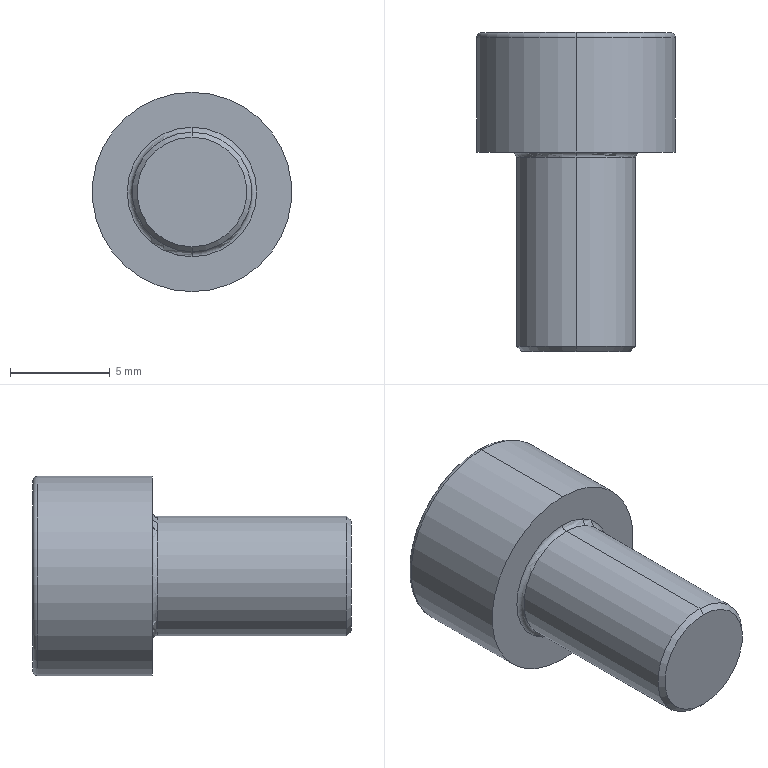Part | STEP file | 1 solid | 20 faces | box 10 x 16 x 10 mm | volume 688.299 mm3 | plane 10 | torus 4 | cylinder 4 | cone 2 | commonest cylinder face diameters 6 x2 10 x2
STEP:
#1=CARTESIAN_POINT('',(0.,-10.,-2.75));
#2=VERTEX_POINT('',#1);
#3=CARTESIAN_POINT('',(0.,-10.,2.75));
#4=VERTEX_POINT('',#3);
#5=CARTESIAN_POINT('',(0.,-10.,0.));
#6=DIRECTION('',(0.,-1.,0.));
#7=DIRECTION('',(0.,0.,-1.));
#8=AXIS2_PLACEMENT_3D('',#5,#6,#7);
#9=CIRCLE('',#8,2.75);
#10=EDGE_CURVE('',#2,#4,#9,.T.);
#11=ORIENTED_EDGE('',*,*,#10,.F.);
#12=CARTESIAN_POINT('',(0.,-9.75,-3.));
#13=VERTEX_POINT('',#12);
#14=CARTESIAN_POINT('',(0.,-10.,-2.75));
#15=DIRECTION('',(0.,0.7071,-0.7071));
#16=VECTOR('',#15,1000.);
#17=LINE('',#14,#16);
#18=EDGE_CURVE('',#2,#13,#17,.T.);
#19=ORIENTED_EDGE('',*,*,#18,.T.);
#20=CARTESIAN_POINT('',(0.,-9.75,3.));
#21=VERTEX_POINT('',#20);
#22=CARTESIAN_POINT('',(0.,-9.75,0.));
#23=DIRECTION('',(0.,1.,0.));
#24=DIRECTION('',(0.,0.,-1.));
#25=AXIS2_PLACEMENT_3D('',#22,#23,#24);
#26=CIRCLE('',#25,3.);
#27=EDGE_CURVE('',#21,#13,#26,.T.);
#28=ORIENTED_EDGE('',*,*,#27,.F.);
#29=CARTESIAN_POINT('',(0.,-10.,2.75));
#30=DIRECTION('',(0.,0.7071,0.7071));
#31=VECTOR('',#30,1000.);
#32=LINE('',#29,#31);
#33=EDGE_CURVE('',#4,#21,#32,.T.);
#34=ORIENTED_EDGE('',*,*,#33,.F.);
#35=EDGE_LOOP('',(#11,#19,#28,#34));
#36=FACE_OUTER_BOUND('',#35,.T.);
#37=CARTESIAN_POINT('',(0.,-10.,0.));
#38=DIRECTION('',(0.,1.,0.));
#39=DIRECTION('',(0.,0.,1.));
#40=AXIS2_PLACEMENT_3D('',#37,#38,#39);
#41=CONICAL_SURFACE('',#40,2.75,0.7854);
#42=ADVANCED_FACE('',(#36),#41,.T.);
#43=CARTESIAN_POINT('',(0.,5.75,-5.));
#44=VERTEX_POINT('',#43);
#45=CARTESIAN_POINT('',(0.,5.75,5.));
#46=VERTEX_POINT('',#45);
#47=CARTESIAN_POINT('',(0.,5.75,0.));
#48=DIRECTION('',(0.,-1.,0.));
#49=DIRECTION('',(0.,0.,1.));
#50=AXIS2_PLACEMENT_3D('',#47,#48,#49);
#51=CIRCLE('',#50,5.);
#52=EDGE_CURVE('',#44,#46,#51,.T.);
#53=ORIENTED_EDGE('',*,*,#52,.F.);
#54=CARTESIAN_POINT('',(0.,6.,-4.75));
#55=VERTEX_POINT('',#54);
#56=CARTESIAN_POINT('',(0.,5.75,-4.75));
#57=DIRECTION('',(1.,0.,0.));
#58=DIRECTION('',(0.,0.,-1.));
#59=AXIS2_PLACEMENT_3D('',#56,#57,#58);
#60=CIRCLE('',#59,0.25);
#61=EDGE_CURVE('',#44,#55,#60,.T.);
#62=ORIENTED_EDGE('',*,*,#61,.T.);
#63=CARTESIAN_POINT('',(0.,6.,4.75));
#64=VERTEX_POINT('',#63);
#65=CARTESIAN_POINT('',(0.,6.,0.));
#66=DIRECTION('',(0.,1.,0.));
#67=DIRECTION('',(0.,0.,1.));
#68=AXIS2_PLACEMENT_3D('',#65,#66,#67);
#69=CIRCLE('',#68,4.75);
#70=EDGE_CURVE('',#64,#55,#69,.T.);
#71=ORIENTED_EDGE('',*,*,#70,.F.);
#72=CARTESIAN_POINT('',(0.,5.75,4.75));
#73=DIRECTION('',(-1.,0.,0.));
#74=DIRECTION('',(0.,0.,1.));
#75=AXIS2_PLACEMENT_3D('',#72,#73,#74);
#76=CIRCLE('',#75,0.25);
#77=EDGE_CURVE('',#46,#64,#76,.T.);
#78=ORIENTED_EDGE('',*,*,#77,.F.);
#79=EDGE_LOOP('',(#53,#62,#71,#78));
#80=FACE_OUTER_BOUND('',#79,.T.);
#81=CARTESIAN_POINT('',(0.,5.75,0.));
#82=DIRECTION('',(0.,1.,0.));
#83=DIRECTION('',(0.,0.,1.));
#84=AXIS2_PLACEMENT_3D('',#81,#82,#83);
#85=TOROIDAL_SURFACE('',#84,4.75,0.25);
#86=ADVANCED_FACE('',(#80),#85,.T.);
#87=CARTESIAN_POINT('',(0.,-0.25,3.));
#88=VERTEX_POINT('',#87);
#89=CARTESIAN_POINT('',(0.,-0.25,-3.));
#90=VERTEX_POINT('',#89);
#91=CARTESIAN_POINT('',(0.,-0.25,0.));
#92=DIRECTION('',(0.,-1.,0.));
#93=DIRECTION('',(0.,0.,-1.));
#94=AXIS2_PLACEMENT_3D('',#91,#92,#93);
#95=CIRCLE('',#94,3.);
#96=EDGE_CURVE('',#88,#90,#95,.T.);
#97=ORIENTED_EDGE('',*,*,#96,.F.);
#98=CARTESIAN_POINT('',(0.,0.,3.25));
#99=VERTEX_POINT('',#98);
#100=CARTESIAN_POINT('',(0.,-0.25,3.25));
#101=DIRECTION('',(1.,0.,0.));
#102=DIRECTION('',(0.,0.,-1.));
#103=AXIS2_PLACEMENT_3D('',#100,#101,#102);
#104=CIRCLE('',#103,0.25);
#105=EDGE_CURVE('',#88,#99,#104,.T.);
#106=ORIENTED_EDGE('',*,*,#105,.T.);
#107=CARTESIAN_POINT('',(0.,0.,-3.25));
#108=VERTEX_POINT('',#107);
#109=CARTESIAN_POINT('',(0.,0.,0.));
#110=DIRECTION('',(0.,1.,0.));
#111=DIRECTION('',(0.,0.,-1.));
#112=AXIS2_PLACEMENT_3D('',#109,#110,#111);
#113=CIRCLE('',#112,3.25);
#114=EDGE_CURVE('',#108,#99,#113,.T.);
#115=ORIENTED_EDGE('',*,*,#114,.F.);
#116=CARTESIAN_POINT('',(0.,-0.25,-3.25));
#117=DIRECTION('',(-1.,0.,0.));
#118=DIRECTION('',(0.,0.,1.));
#119=AXIS2_PLACEMENT_3D('',#116,#117,#118);
#120=CIRCLE('',#119,0.25);
#121=EDGE_CURVE('',#90,#108,#120,.T.);
#122=ORIENTED_EDGE('',*,*,#121,.F.);
#123=EDGE_LOOP('',(#97,#106,#115,#122));
#124=FACE_OUTER_BOUND('',#123,.T.);
#125=CARTESIAN_POINT('',(0.,-0.25,0.));
#126=DIRECTION('',(0.,-1.,0.));
#127=DIRECTION('',(0.,0.,-1.));
#128=AXIS2_PLACEMENT_3D('',#125,#126,#127);
#129=TOROIDAL_SURFACE('',#128,3.25,0.25);
#130=ADVANCED_FACE('',(#124),#129,.F.);
#131=CARTESIAN_POINT('',(0.,-0.25,0.));
#132=DIRECTION('',(0.,-1.,0.));
#133=DIRECTION('',(0.,0.,-1.));
#134=AXIS2_PLACEMENT_3D('',#131,#132,#133);
#135=CIRCLE('',#134,3.);
#136=EDGE_CURVE('',#90,#88,#135,.T.);
#137=ORIENTED_EDGE('',*,*,#136,.T.);
#138=CARTESIAN_POINT('',(0.,0.,3.));
#139=DIRECTION('',(0.,-1.,0.));
#140=VECTOR('',#139,1000.);
#141=LINE('',#138,#140);
#142=EDGE_CURVE('',#88,#21,#141,.T.);
#143=ORIENTED_EDGE('',*,*,#142,.T.);
#144=ORIENTED_EDGE('',*,*,#27,.T.);
#145=CARTESIAN_POINT('',(0.,0.,-3.));
#146=DIRECTION('',(0.,-1.,0.));
#147=VECTOR('',#146,1000.);
#148=LINE('',#145,#147);
#149=EDGE_CURVE('',#90,#13,#148,.T.);
#150=ORIENTED_EDGE('',*,*,#149,.F.);
#151=EDGE_LOOP('',(#137,#143,#144,#150));
#152=FACE_OUTER_BOUND('',#151,.T.);
#153=CARTESIAN_POINT('',(0.,0.,0.));
#154=DIRECTION('',(0.,-1.,0.));
#155=DIRECTION('',(0.,0.,-1.));
#156=AXIS2_PLACEMENT_3D('',#153,#154,#155);
#157=CYLINDRICAL_SURFACE('',#156,3.);
#158=ADVANCED_FACE('',(#152),#157,.T.);
#159=ORIENTED_EDGE('',*,*,#52,.T.);
#160=CARTESIAN_POINT('',(0.,0.,5.));
#161=VERTEX_POINT('',#160);
#162=CARTESIAN_POINT('',(0.,0.,5.));
#163=DIRECTION('',(0.,-1.,0.));
#164=VECTOR('',#163,1000.);
#165=LINE('',#162,#164);
#166=EDGE_CURVE('',#46,#161,#165,.T.);
#167=ORIENTED_EDGE('',*,*,#166,.T.);
#168=CARTESIAN_POINT('',(0.,0.,-5.));
#169=VERTEX_POINT('',#168);
#170=CARTESIAN_POINT('',(0.,0.,0.));
#171=DIRECTION('',(0.,-1.,0.));
#172=DIRECTION('',(0.,0.,-1.));
#173=AXIS2_PLACEMENT_3D('',#170,#171,#172);
#174=CIRCLE('',#173,5.);
#175=EDGE_CURVE('',#169,#161,#174,.T.);
#176=ORIENTED_EDGE('',*,*,#175,.F.);
#177=CARTESIAN_POINT('',(0.,0.,-5.));
#178=DIRECTION('',(0.,-1.,0.));
#179=VECTOR('',#178,1000.);
#180=LINE('',#177,#179);
#181=EDGE_CURVE('',#44,#169,#180,.T.);
#182=ORIENTED_EDGE('',*,*,#181,.F.);
#183=EDGE_LOOP('',(#159,#167,#176,#182));
#184=FACE_OUTER_BOUND('',#183,.T.);
#185=CARTESIAN_POINT('',(0.,0.,0.));
#186=DIRECTION('',(0.,-1.,0.));
#187=DIRECTION('',(0.,0.,-1.));
#188=AXIS2_PLACEMENT_3D('',#185,#186,#187);
#189=CYLINDRICAL_SURFACE('',#188,5.);
#190=ADVANCED_FACE('',(#184),#189,.T.);
#191=ORIENTED_EDGE('',*,*,#70,.T.);
#192=CARTESIAN_POINT('',(0.,6.,0.));
#193=DIRECTION('',(0.,1.,0.));
#194=DIRECTION('',(0.,0.,1.));
#195=AXIS2_PLACEMENT_3D('',#192,#193,#194);
#196=CIRCLE('',#195,4.75);
#197=EDGE_CURVE('',#55,#64,#196,.T.);
#198=ORIENTED_EDGE('',*,*,#197,.T.);
#199=EDGE_LOOP('',(#191,#198));
#200=FACE_OUTER_BOUND('',#199,.T.);
#201=CARTESIAN_POINT('',(0.,6.,-2.887));
#202=VERTEX_POINT('',#201);
#203=CARTESIAN_POINT('',(-2.5,6.,-1.443));
#204=VERTEX_POINT('',#203);
#205=CARTESIAN_POINT('',(0.,6.,-2.887));
#206=DIRECTION('',(-0.866,0.,0.5));
#207=VECTOR('',#206,1000.);
#208=LINE('',#205,#207);
#209=EDGE_CURVE('',#202,#204,#208,.T.);
#210=ORIENTED_EDGE('',*,*,#209,.F.);
#211=CARTESIAN_POINT('',(2.5,6.,-1.443));
#212=VERTEX_POINT('',#211);
#213=CARTESIAN_POINT('',(2.5,6.,-1.443));
#214=DIRECTION('',(-0.866,0.,-0.5));
#215=VECTOR('',#214,1000.);
#216=LINE('',#213,#215);
#217=EDGE_CURVE('',#212,#202,#216,.T.);
#218=ORIENTED_EDGE('',*,*,#217,.F.);
#219=CARTESIAN_POINT('',(2.5,6.,1.443));
#220=VERTEX_POINT('',#219);
#221=CARTESIAN_POINT('',(2.5,6.,1.443));
#222=DIRECTION('',(0.,0.,-1.));
#223=VECTOR('',#222,1000.);
#224=LINE('',#221,#223);
#225=EDGE_CURVE('',#220,#212,#224,.T.);
#226=ORIENTED_EDGE('',*,*,#225,.F.);
#227=CARTESIAN_POINT('',(0.,6.,2.887));
#228=VERTEX_POINT('',#227);
#229=CARTESIAN_POINT('',(0.,6.,2.887));
#230=DIRECTION('',(0.866,0.,-0.5));
#231=VECTOR('',#230,1000.);
#232=LINE('',#229,#231);
#233=EDGE_CURVE('',#228,#220,#232,.T.);
#234=ORIENTED_EDGE('',*,*,#233,.F.);
#235=CARTESIAN_POINT('',(-2.5,6.,1.443));
#236=VERTEX_POINT('',#235);
#237=CARTESIAN_POINT('',(-2.5,6.,1.443));
#238=DIRECTION('',(0.866,0.,0.5));
#239=VECTOR('',#238,1000.);
#240=LINE('',#237,#239);
#241=EDGE_CURVE('',#236,#228,#240,.T.);
#242=ORIENTED_EDGE('',*,*,#241,.F.);
#243=CARTESIAN_POINT('',(-2.5,6.,-1.443));
#244=DIRECTION('',(0.,0.,1.));
#245=VECTOR('',#244,1000.);
#246=LINE('',#243,#245);
#247=EDGE_CURVE('',#204,#236,#246,.T.);
#248=ORIENTED_EDGE('',*,*,#247,.F.);
#249=EDGE_LOOP('',(#210,#218,#226,#234,#242,#248));
#250=FACE_BOUND('',#249,.T.);
#251=CARTESIAN_POINT('',(0.,6.,0.));
#252=DIRECTION('',(0.,1.,0.));
#253=DIRECTION('',(0.,0.,1.));
#254=AXIS2_PLACEMENT_3D('',#251,#252,#253);
#255=PLANE('',#254);
#256=ADVANCED_FACE('',(#200,#250),#255,.T.);
#257=ORIENTED_EDGE('',*,*,#166,.F.);
#258=CARTESIAN_POINT('',(0.,5.75,0.));
#259=DIRECTION('',(0.,-1.,0.));
#260=DIRECTION('',(0.,0.,1.));
#261=AXIS2_PLACEMENT_3D('',#258,#259,#260);
#262=CIRCLE('',#261,5.);
#263=EDGE_CURVE('',#46,#44,#262,.T.);
#264=ORIENTED_EDGE('',*,*,#263,.T.);
#265=ORIENTED_EDGE('',*,*,#181,.T.);
#266=CARTESIAN_POINT('',(0.,0.,0.));
#267=DIRECTION('',(0.,-1.,0.));
#268=DIRECTION('',(0.,0.,-1.));
#269=AXIS2_PLACEMENT_3D('',#266,#267,#268);
#270=CIRCLE('',#269,5.);
#271=EDGE_CURVE('',#161,#169,#270,.T.);
#272=ORIENTED_EDGE('',*,*,#271,.F.);
#273=EDGE_LOOP('',(#257,#264,#265,#272));
#274=FACE_OUTER_BOUND('',#273,.T.);
#275=CARTESIAN_POINT('',(0.,0.,0.));
#276=DIRECTION('',(0.,-1.,0.));
#277=DIRECTION('',(0.,0.,-1.));
#278=AXIS2_PLACEMENT_3D('',#275,#276,#277);
#279=CYLINDRICAL_SURFACE('',#278,5.);
#280=ADVANCED_FACE('',(#274),#279,.T.);
#281=ORIENTED_EDGE('',*,*,#114,.T.);
#282=CARTESIAN_POINT('',(0.,0.,0.));
#283=DIRECTION('',(0.,1.,0.));
#284=DIRECTION('',(0.,0.,-1.));
#285=AXIS2_PLACEMENT_3D('',#282,#283,#284);
#286=CIRCLE('',#285,3.25);
#287=EDGE_CURVE('',#99,#108,#286,.T.);
#288=ORIENTED_EDGE('',*,*,#287,.T.);
#289=EDGE_LOOP('',(#281,#288));
#290=FACE_BOUND('',#289,.T.);
#291=ORIENTED_EDGE('',*,*,#175,.T.);
#292=ORIENTED_EDGE('',*,*,#271,.T.);
#293=EDGE_LOOP('',(#291,#292));
#294=FACE_OUTER_BOUND('',#293,.T.);
#295=CARTESIAN_POINT('',(5.,0.,0.));
#296=DIRECTION('',(0.,-1.,0.));
#297=DIRECTION('',(0.,0.,-1.));
#298=AXIS2_PLACEMENT_3D('',#295,#296,#297);
#299=PLANE('',#298);
#300=ADVANCED_FACE('',(#290,#294),#299,.T.);
#301=ORIENTED_EDGE('',*,*,#142,.F.);
#302=ORIENTED_EDGE('',*,*,#96,.T.);
#303=ORIENTED_EDGE('',*,*,#149,.T.);
#304=CARTESIAN_POINT('',(0.,-9.75,0.));
#305=DIRECTION('',(0.,1.,0.));
#306=DIRECTION('',(0.,0.,-1.));
#307=AXIS2_PLACEMENT_3D('',#304,#305,#306);
#308=CIRCLE('',#307,3.);
#309=EDGE_CURVE('',#13,#21,#308,.T.);
#310=ORIENTED_EDGE('',*,*,#309,.T.);
#311=EDGE_LOOP('',(#301,#302,#303,#310));
#312=FACE_OUTER_BOUND('',#311,.T.);
#313=CARTESIAN_POINT('',(0.,0.,0.));
#314=DIRECTION('',(0.,-1.,0.));
#315=DIRECTION('',(0.,0.,-1.));
#316=AXIS2_PLACEMENT_3D('',#313,#314,#315);
#317=CYLINDRICAL_SURFACE('',#316,3.);
#318=ADVANCED_FACE('',(#312),#317,.T.);
#319=CARTESIAN_POINT('',(0.,-10.,0.));
#320=DIRECTION('',(0.,-1.,0.));
#321=DIRECTION('',(0.,0.,-1.));
#322=AXIS2_PLACEMENT_3D('',#319,#320,#321);
#323=CIRCLE('',#322,2.75);
#324=EDGE_CURVE('',#4,#2,#323,.T.);
#325=ORIENTED_EDGE('',*,*,#324,.T.);
#326=ORIENTED_EDGE('',*,*,#10,.T.);
#327=EDGE_LOOP('',(#325,#326));
#328=FACE_OUTER_BOUND('',#327,.T.);
#329=CARTESIAN_POINT('',(3.,-10.,0.));
#330=DIRECTION('',(0.,-1.,0.));
#331=DIRECTION('',(0.,0.,-1.));
#332=AXIS2_PLACEMENT_3D('',#329,#330,#331);
#333=PLANE('',#332);
#334=ADVANCED_FACE('',(#328),#333,.T.);
#335=ORIENTED_EDGE('',*,*,#209,.T.);
#336=CARTESIAN_POINT('',(-2.5,3.,-1.443));
#337=VERTEX_POINT('',#336);
#338=CARTESIAN_POINT('',(-2.5,3.,-1.443));
#339=DIRECTION('',(0.,1.,0.));
#340=VECTOR('',#339,1000.);
#341=LINE('',#338,#340);
#342=EDGE_CURVE('',#337,#204,#341,.T.);
#343=ORIENTED_EDGE('',*,*,#342,.F.);
#344=CARTESIAN_POINT('',(0.,3.,-2.887));
#345=VERTEX_POINT('',#344);
#346=CARTESIAN_POINT('',(0.,3.,-2.887));
#347=DIRECTION('',(-0.866,0.,0.5));
#348=VECTOR('',#347,1000.);
#349=LINE('',#346,#348);
#350=EDGE_CURVE('',#345,#337,#349,.T.);
#351=ORIENTED_EDGE('',*,*,#350,.F.);
#352=CARTESIAN_POINT('',(0.,3.,-2.887));
#353=DIRECTION('',(0.,1.,0.));
#354=VECTOR('',#353,1000.);
#355=LINE('',#352,#354);
#356=EDGE_CURVE('',#345,#202,#355,.T.);
#357=ORIENTED_EDGE('',*,*,#356,.T.);
#358=EDGE_LOOP('',(#335,#343,#351,#357));
#359=FACE_OUTER_BOUND('',#358,.T.);
#360=CARTESIAN_POINT('',(0.,3.,-2.887));
#361=DIRECTION('',(-0.5,0.,-0.866));
#362=DIRECTION('',(-0.866,0.,0.5));
#363=AXIS2_PLACEMENT_3D('',#360,#361,#362);
#364=PLANE('',#363);
#365=ADVANCED_FACE('',(#359),#364,.F.);
#366=ORIENTED_EDGE('',*,*,#217,.T.);
#367=ORIENTED_EDGE('',*,*,#356,.F.);
#368=CARTESIAN_POINT('',(2.5,3.,-1.443));
#369=VERTEX_POINT('',#368);
#370=CARTESIAN_POINT('',(2.5,3.,-1.443));
#371=DIRECTION('',(-0.866,0.,-0.5));
#372=VECTOR('',#371,1000.);
#373=LINE('',#370,#372);
#374=EDGE_CURVE('',#369,#345,#373,.T.);
#375=ORIENTED_EDGE('',*,*,#374,.F.);
#376=CARTESIAN_POINT('',(2.5,3.,-1.443));
#377=DIRECTION('',(0.,1.,0.));
#378=VECTOR('',#377,1000.);
#379=LINE('',#376,#378);
#380=EDGE_CURVE('',#369,#212,#379,.T.);
#381=ORIENTED_EDGE('',*,*,#380,.T.);
#382=EDGE_LOOP('',(#366,#367,#375,#381));
#383=FACE_OUTER_BOUND('',#382,.T.);
#384=CARTESIAN_POINT('',(2.5,3.,-1.443));
#385=DIRECTION('',(0.5,0.,-0.866));
#386=DIRECTION('',(-0.866,0.,-0.5));
#387=AXIS2_PLACEMENT_3D('',#384,#385,#386);
#388=PLANE('',#387);
#389=ADVANCED_FACE('',(#383),#388,.F.);
#390=ORIENTED_EDGE('',*,*,#225,.T.);
#391=ORIENTED_EDGE('',*,*,#380,.F.);
#392=CARTESIAN_POINT('',(2.5,3.,1.443));
#393=VERTEX_POINT('',#392);
#394=CARTESIAN_POINT('',(2.5,3.,1.443));
#395=DIRECTION('',(0.,0.,-1.));
#396=VECTOR('',#395,1000.);
#397=LINE('',#394,#396);
#398=EDGE_CURVE('',#393,#369,#397,.T.);
#399=ORIENTED_EDGE('',*,*,#398,.F.);
#400=CARTESIAN_POINT('',(2.5,3.,1.443));
#401=DIRECTION('',(0.,1.,0.));
#402=VECTOR('',#401,1000.);
#403=LINE('',#400,#402);
#404=EDGE_CURVE('',#393,#220,#403,.T.);
#405=ORIENTED_EDGE('',*,*,#404,.T.);
#406=EDGE_LOOP('',(#390,#391,#399,#405));
#407=FACE_OUTER_BOUND('',#406,.T.);
#408=CARTESIAN_POINT('',(2.5,3.,1.443));
#409=DIRECTION('',(1.,0.,0.));
#410=DIRECTION('',(0.,0.,-1.));
#411=AXIS2_PLACEMENT_3D('',#408,#409,#410);
#412=PLANE('',#411);
#413=ADVANCED_FACE('',(#407),#412,.F.);
#414=ORIENTED_EDGE('',*,*,#233,.T.);
#415=ORIENTED_EDGE('',*,*,#404,.F.);
#416=CARTESIAN_POINT('',(0.,3.,2.887));
#417=VERTEX_POINT('',#416);
#418=CARTESIAN_POINT('',(0.,3.,2.887));
#419=DIRECTION('',(0.866,0.,-0.5));
#420=VECTOR('',#419,1000.);
#421=LINE('',#418,#420);
#422=EDGE_CURVE('',#417,#393,#421,.T.);
#423=ORIENTED_EDGE('',*,*,#422,.F.);
#424=CARTESIAN_POINT('',(0.,3.,2.887));
#425=DIRECTION('',(0.,1.,0.));
#426=VECTOR('',#425,1000.);
#427=LINE('',#424,#426);
#428=EDGE_CURVE('',#417,#228,#427,.T.);
#429=ORIENTED_EDGE('',*,*,#428,.T.);
#430=EDGE_LOOP('',(#414,#415,#423,#429));
#431=FACE_OUTER_BOUND('',#430,.T.);
#432=CARTESIAN_POINT('',(0.,3.,2.887));
#433=DIRECTION('',(0.5,0.,0.866));
#434=DIRECTION('',(0.866,0.,-0.5));
#435=AXIS2_PLACEMENT_3D('',#432,#433,#434);
#436=PLANE('',#435);
#437=ADVANCED_FACE('',(#431),#436,.F.);
#438=ORIENTED_EDGE('',*,*,#241,.T.);
#439=ORIENTED_EDGE('',*,*,#428,.F.);
#440=CARTESIAN_POINT('',(-2.5,3.,1.443));
#441=VERTEX_POINT('',#440);
#442=CARTESIAN_POINT('',(-2.5,3.,1.443));
#443=DIRECTION('',(0.866,0.,0.5));
#444=VECTOR('',#443,1000.);
#445=LINE('',#442,#444);
#446=EDGE_CURVE('',#441,#417,#445,.T.);
#447=ORIENTED_EDGE('',*,*,#446,.F.);
#448=CARTESIAN_POINT('',(-2.5,3.,1.443));
#449=DIRECTION('',(0.,1.,0.));
#450=VECTOR('',#449,1000.);
#451=LINE('',#448,#450);
#452=EDGE_CURVE('',#441,#236,#451,.T.);
#453=ORIENTED_EDGE('',*,*,#452,.T.);
#454=EDGE_LOOP('',(#438,#439,#447,#453));
#455=FACE_OUTER_BOUND('',#454,.T.);
#456=CARTESIAN_POINT('',(-2.5,3.,1.443));
#457=DIRECTION('',(-0.5,0.,0.866));
#458=DIRECTION('',(0.866,0.,0.5));
#459=AXIS2_PLACEMENT_3D('',#456,#457,#458);
#460=PLANE('',#459);
#461=ADVANCED_FACE('',(#455),#460,.F.);
#462=ORIENTED_EDGE('',*,*,#247,.T.);
#463=ORIENTED_EDGE('',*,*,#452,.F.);
#464=CARTESIAN_POINT('',(-2.5,3.,-1.443));
#465=DIRECTION('',(0.,0.,1.));
#466=VECTOR('',#465,1000.);
#467=LINE('',#464,#466);
#468=EDGE_CURVE('',#337,#441,#467,.T.);
#469=ORIENTED_EDGE('',*,*,#468,.F.);
#470=ORIENTED_EDGE('',*,*,#342,.T.);
#471=EDGE_LOOP('',(#462,#463,#469,#470));
#472=FACE_OUTER_BOUND('',#471,.T.);
#473=CARTESIAN_POINT('',(-2.5,3.,-1.443));
#474=DIRECTION('',(-1.,0.,0.));
#475=DIRECTION('',(0.,0.,1.));
#476=AXIS2_PLACEMENT_3D('',#473,#474,#475);
#477=PLANE('',#476);
#478=ADVANCED_FACE('',(#472),#477,.F.);
#479=ORIENTED_EDGE('',*,*,#350,.T.);
#480=ORIENTED_EDGE('',*,*,#468,.T.);
#481=ORIENTED_EDGE('',*,*,#446,.T.);
#482=ORIENTED_EDGE('',*,*,#422,.T.);
#483=ORIENTED_EDGE('',*,*,#398,.T.);
#484=ORIENTED_EDGE('',*,*,#374,.T.);
#485=EDGE_LOOP('',(#479,#480,#481,#482,#483,#484));
#486=FACE_OUTER_BOUND('',#485,.T.);
#487=CARTESIAN_POINT('',(0.,3.,0.));
#488=DIRECTION('',(0.,1.,0.));
#489=DIRECTION('',(0.,0.,1.));
#490=AXIS2_PLACEMENT_3D('',#487,#488,#489);
#491=PLANE('',#490);
#492=ADVANCED_FACE('',(#486),#491,.T.);
#493=ORIENTED_EDGE('',*,*,#105,.F.);
#494=ORIENTED_EDGE('',*,*,#136,.F.);
#495=ORIENTED_EDGE('',*,*,#121,.T.);
#496=ORIENTED_EDGE('',*,*,#287,.F.);
#497=EDGE_LOOP('',(#493,#494,#495,#496));
#498=FACE_OUTER_BOUND('',#497,.T.);
#499=CARTESIAN_POINT('',(0.,-0.25,0.));
#500=DIRECTION('',(0.,-1.,0.));
#501=DIRECTION('',(0.,0.,-1.));
#502=AXIS2_PLACEMENT_3D('',#499,#500,#501);
#503=TOROIDAL_SURFACE('',#502,3.25,0.25);
#504=ADVANCED_FACE('',(#498),#503,.F.);
#505=ORIENTED_EDGE('',*,*,#61,.F.);
#506=ORIENTED_EDGE('',*,*,#263,.F.);
#507=ORIENTED_EDGE('',*,*,#77,.T.);
#508=ORIENTED_EDGE('',*,*,#197,.F.);
#509=EDGE_LOOP('',(#505,#506,#507,#508));
#510=FACE_OUTER_BOUND('',#509,.T.);
#511=CARTESIAN_POINT('',(0.,5.75,0.));
#512=DIRECTION('',(0.,1.,0.));
#513=DIRECTION('',(0.,0.,1.));
#514=AXIS2_PLACEMENT_3D('',#511,#512,#513);
#515=TOROIDAL_SURFACE('',#514,4.75,0.25);
#516=ADVANCED_FACE('',(#510),#515,.T.);
#517=ORIENTED_EDGE('',*,*,#18,.F.);
#518=ORIENTED_EDGE('',*,*,#324,.F.);
#519=ORIENTED_EDGE('',*,*,#33,.T.);
#520=ORIENTED_EDGE('',*,*,#309,.F.);
#521=EDGE_LOOP('',(#517,#518,#519,#520));
#522=FACE_OUTER_BOUND('',#521,.T.);
#523=CARTESIAN_POINT('',(0.,-10.,0.));
#524=DIRECTION('',(0.,1.,0.));
#525=DIRECTION('',(0.,0.,1.));
#526=AXIS2_PLACEMENT_3D('',#523,#524,#525);
#527=CONICAL_SURFACE('',#526,2.75,0.7854);
#528=ADVANCED_FACE('',(#522),#527,.T.);
#529=CLOSED_SHELL('',(#42,#86,#130,#158,#190,#256,#280,#300,#318,#334,#365,#389,#413,#437,#461,#478,#492,#504,#516,#528));
#530=MANIFOLD_SOLID_BREP('',#529);
#531=CARTESIAN_POINT('',(0.,0.,0.));
#532=DIRECTION('',(0.,0.,1.));
#533=DIRECTION('',(1.,0.,0.));
#534=AXIS2_PLACEMENT_3D('',#531,#532,#533);
#535=(LENGTH_UNIT()NAMED_UNIT(*)SI_UNIT(.MILLI.,.METRE.));
#536=UNCERTAINTY_MEASURE_WITH_UNIT(LENGTH_MEASURE(0.00001),#535,'','');
#537=(NAMED_UNIT(*)PLANE_ANGLE_UNIT()SI_UNIT($,.RADIAN.));
#538=(NAMED_UNIT(*)SI_UNIT($,.STERADIAN.)SOLID_ANGLE_UNIT());
#539=(GEOMETRIC_REPRESENTATION_CONTEXT(3)GLOBAL_UNCERTAINTY_ASSIGNED_CONTEXT((#536))GLOBAL_UNIT_ASSIGNED_CONTEXT((#535,#537,#538))REPRESENTATION_CONTEXT('',''));
#540=ADVANCED_BREP_SHAPE_REPRESENTATION('',(#530,#534),#539);